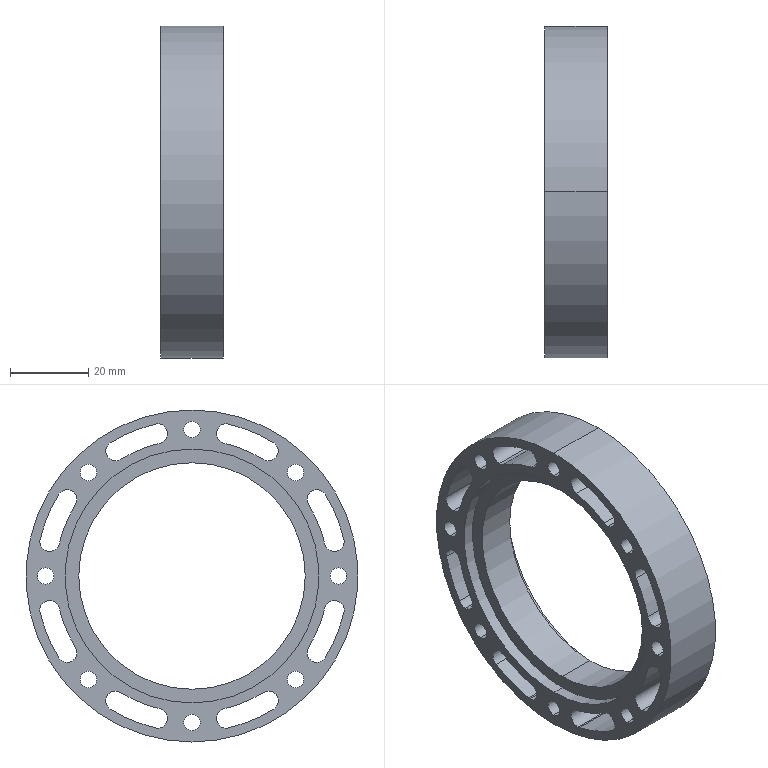Part | SolidWorks | features ICE 1, Revolution 1 | 1 solid | 68 faces | box 16 x 85 x 85 mm | volume 32635 mm3 | cylinder 64 | plane 4 | commonest cylinder face diameters 5 x24 4.2 x16 70 x8 80 x8 65 x4 58 x2